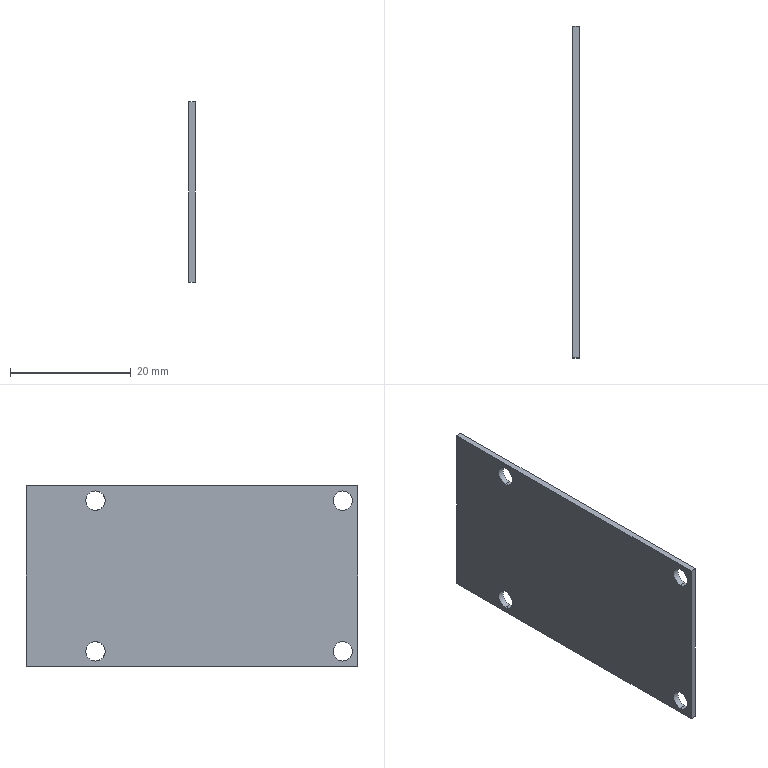Part | STEP file | RJ-GRBT-V1_1-221125 | 1 solid | 14 faces | box 1 x 55 x 30 mm | volume 1618 mm3 | cylinder 8 | plane 6 | commonest cylinder face diameters 3.2 x8
STEP:
#1=CARTESIAN_POINT('',(0.,0.,0.));
#2=DIRECTION('',(0.,0.,1.));
#3=DIRECTION('',(1.,0.,0.));
#4=AXIS2_PLACEMENT_3D('',#1,#2,#3);
#5=CARTESIAN_POINT('',(658.041,4225.2,279.644));
#6=VERTEX_POINT('',#5);
#7=CARTESIAN_POINT('',(658.041,4225.2,309.644));
#8=VERTEX_POINT('',#7);
#9=CARTESIAN_POINT('',(658.041,4225.2,279.644));
#10=DIRECTION('',(0.,0.,1.));
#11=VECTOR('',#10,1.);
#12=LINE('',#9,#11);
#13=CARTESIAN_POINT('',(659.041,4225.2,309.644));
#14=DIRECTION('',(0.,1.,0.));
#15=DIRECTION('',(0.,0.,1.));
#16=AXIS2_PLACEMENT_3D('',#13,#14,#15);
#17=PLANE('',#16);
#18=CARTESIAN_POINT('',(-30.,-1.));
#19=DIRECTION('',(1.,0.));
#20=VECTOR('',#19,1.);
#21=LINE('',#18,#20);
#22=(GEOMETRIC_REPRESENTATION_CONTEXT(2)PARAMETRIC_REPRESENTATION_CONTEXT()REPRESENTATION_CONTEXT('',''));
#23=DEFINITIONAL_REPRESENTATION('',(#21),#22);
#24=PCURVE('',#17,#23);
#25=CARTESIAN_POINT('',(658.041,4227.7,282.144));
#26=DIRECTION('',(1.,0.,0.));
#27=DIRECTION('',(0.,0.,-1.));
#28=AXIS2_PLACEMENT_3D('',#25,#26,#27);
#29=PLANE('',#28);
#30=CARTESIAN_POINT('',(2.5,-2.5));
#31=DIRECTION('',(-1.,0.));
#32=VECTOR('',#31,1.);
#33=LINE('',#30,#32);
#34=(GEOMETRIC_REPRESENTATION_CONTEXT(2)PARAMETRIC_REPRESENTATION_CONTEXT()REPRESENTATION_CONTEXT('',''));
#35=DEFINITIONAL_REPRESENTATION('',(#33),#34);
#36=PCURVE('',#29,#35);
#37=SURFACE_CURVE('',#12,(#24,#36),.PCURVE_S1.);
#38=EDGE_CURVE('',#6,#8,#37,.T.);
#39=ORIENTED_EDGE('',*,*,#38,.T.);
#40=CARTESIAN_POINT('',(659.041,4225.2,309.644));
#41=VERTEX_POINT('',#40);
#42=CARTESIAN_POINT('',(658.041,4225.2,309.644));
#43=DIRECTION('',(1.,0.,0.));
#44=VECTOR('',#43,1.);
#45=LINE('',#42,#44);
#46=CARTESIAN_POINT('',(0.,-1.));
#47=DIRECTION('',(0.,1.));
#48=VECTOR('',#47,1.);
#49=LINE('',#46,#48);
#50=(GEOMETRIC_REPRESENTATION_CONTEXT(2)PARAMETRIC_REPRESENTATION_CONTEXT()REPRESENTATION_CONTEXT('',''));
#51=DEFINITIONAL_REPRESENTATION('',(#49),#50);
#52=PCURVE('',#17,#51);
#53=CARTESIAN_POINT('',(659.041,4280.2,309.644));
#54=DIRECTION('',(0.,0.,-1.));
#55=DIRECTION('',(-1.,0.,0.));
#56=AXIS2_PLACEMENT_3D('',#53,#54,#55);
#57=PLANE('',#56);
#58=CARTESIAN_POINT('',(1.,-55.));
#59=DIRECTION('',(-1.,0.));
#60=VECTOR('',#59,1.);
#61=LINE('',#58,#60);
#62=(GEOMETRIC_REPRESENTATION_CONTEXT(2)PARAMETRIC_REPRESENTATION_CONTEXT()REPRESENTATION_CONTEXT('',''));
#63=DEFINITIONAL_REPRESENTATION('',(#61),#62);
#64=PCURVE('',#57,#63);
#65=SURFACE_CURVE('',#45,(#52,#64),.PCURVE_S1.);
#66=EDGE_CURVE('',#8,#41,#65,.T.);
#67=ORIENTED_EDGE('',*,*,#66,.T.);
#68=CARTESIAN_POINT('',(659.041,4225.2,279.644));
#69=VERTEX_POINT('',#68);
#70=CARTESIAN_POINT('',(659.041,4225.2,279.644));
#71=DIRECTION('',(0.,0.,1.));
#72=VECTOR('',#71,1.);
#73=LINE('',#70,#72);
#74=CARTESIAN_POINT('',(-30.,0.));
#75=DIRECTION('',(1.,0.));
#76=VECTOR('',#75,1.);
#77=LINE('',#74,#76);
#78=(GEOMETRIC_REPRESENTATION_CONTEXT(2)PARAMETRIC_REPRESENTATION_CONTEXT()REPRESENTATION_CONTEXT('',''));
#79=DEFINITIONAL_REPRESENTATION('',(#77),#78);
#80=PCURVE('',#17,#79);
#81=CARTESIAN_POINT('',(659.041,4227.7,282.144));
#82=DIRECTION('',(1.,0.,0.));
#83=DIRECTION('',(0.,0.,-1.));
#84=AXIS2_PLACEMENT_3D('',#81,#82,#83);
#85=PLANE('',#84);
#86=CARTESIAN_POINT('',(2.5,-2.5));
#87=DIRECTION('',(-1.,0.));
#88=VECTOR('',#87,1.);
#89=LINE('',#86,#88);
#90=(GEOMETRIC_REPRESENTATION_CONTEXT(2)PARAMETRIC_REPRESENTATION_CONTEXT()REPRESENTATION_CONTEXT('',''));
#91=DEFINITIONAL_REPRESENTATION('',(#89),#90);
#92=PCURVE('',#85,#91);
#93=SURFACE_CURVE('',#73,(#80,#92),.PCURVE_S1.);
#94=EDGE_CURVE('',#69,#41,#93,.T.);
#95=ORIENTED_EDGE('',*,*,#94,.F.);
#96=CARTESIAN_POINT('',(658.041,4225.2,279.644));
#97=DIRECTION('',(1.,0.,0.));
#98=VECTOR('',#97,1.);
#99=LINE('',#96,#98);
#100=CARTESIAN_POINT('',(-30.,-1.));
#101=DIRECTION('',(0.,1.));
#102=VECTOR('',#101,1.);
#103=LINE('',#100,#102);
#104=(GEOMETRIC_REPRESENTATION_CONTEXT(2)PARAMETRIC_REPRESENTATION_CONTEXT()REPRESENTATION_CONTEXT('',''));
#105=DEFINITIONAL_REPRESENTATION('',(#103),#104);
#106=PCURVE('',#17,#105);
#107=CARTESIAN_POINT('',(659.041,4225.2,279.644));
#108=DIRECTION('',(0.,0.,1.));
#109=DIRECTION('',(1.,0.,0.));
#110=AXIS2_PLACEMENT_3D('',#107,#108,#109);
#111=PLANE('',#110);
#112=CARTESIAN_POINT('',(-1.,0.));
#113=DIRECTION('',(1.,0.));
#114=VECTOR('',#113,1.);
#115=LINE('',#112,#114);
#116=(GEOMETRIC_REPRESENTATION_CONTEXT(2)PARAMETRIC_REPRESENTATION_CONTEXT()REPRESENTATION_CONTEXT('',''));
#117=DEFINITIONAL_REPRESENTATION('',(#115),#116);
#118=PCURVE('',#111,#117);
#119=SURFACE_CURVE('',#99,(#106,#118),.PCURVE_S1.);
#120=EDGE_CURVE('',#6,#69,#119,.T.);
#121=ORIENTED_EDGE('',*,*,#120,.F.);
#122=EDGE_LOOP('',(#39,#67,#95,#121));
#123=FACE_BOUND('',#122,.F.);
#124=ADVANCED_FACE('',(#123),#17,.F.);
#125=ORIENTED_EDGE('',*,*,#38,.F.);
#126=CARTESIAN_POINT('',(658.041,4280.2,279.644));
#127=VERTEX_POINT('',#126);
#128=CARTESIAN_POINT('',(658.041,4280.2,279.644));
#129=DIRECTION('',(0.,-1.,0.));
#130=VECTOR('',#129,1.);
#131=LINE('',#128,#130);
#132=CARTESIAN_POINT('',(2.5,52.5));
#133=DIRECTION('',(0.,-1.));
#134=VECTOR('',#133,1.);
#135=LINE('',#132,#134);
#136=(GEOMETRIC_REPRESENTATION_CONTEXT(2)PARAMETRIC_REPRESENTATION_CONTEXT()REPRESENTATION_CONTEXT('',''));
#137=DEFINITIONAL_REPRESENTATION('',(#135),#136);
#138=PCURVE('',#29,#137);
#139=CARTESIAN_POINT('',(-1.,55.));
#140=DIRECTION('',(0.,-1.));
#141=VECTOR('',#140,1.);
#142=LINE('',#139,#141);
#143=(GEOMETRIC_REPRESENTATION_CONTEXT(2)PARAMETRIC_REPRESENTATION_CONTEXT()REPRESENTATION_CONTEXT('',''));
#144=DEFINITIONAL_REPRESENTATION('',(#142),#143);
#145=PCURVE('',#111,#144);
#146=SURFACE_CURVE('',#131,(#138,#145),.PCURVE_S1.);
#147=EDGE_CURVE('',#127,#6,#146,.T.);
#148=ORIENTED_EDGE('',*,*,#147,.F.);
#149=CARTESIAN_POINT('',(658.041,4280.2,309.644));
#150=VERTEX_POINT('',#149);
#151=CARTESIAN_POINT('',(658.041,4280.2,309.644));
#152=DIRECTION('',(0.,0.,-1.));
#153=VECTOR('',#152,1.);
#154=LINE('',#151,#153);
#155=CARTESIAN_POINT('',(-27.5,52.5));
#156=DIRECTION('',(1.,0.));
#157=VECTOR('',#156,1.);
#158=LINE('',#155,#157);
#159=(GEOMETRIC_REPRESENTATION_CONTEXT(2)PARAMETRIC_REPRESENTATION_CONTEXT()REPRESENTATION_CONTEXT('',''));
#160=DEFINITIONAL_REPRESENTATION('',(#158),#159);
#161=PCURVE('',#29,#160);
#162=CARTESIAN_POINT('',(659.041,4280.2,279.644));
#163=DIRECTION('',(0.,-1.,0.));
#164=DIRECTION('',(0.,0.,-1.));
#165=AXIS2_PLACEMENT_3D('',#162,#163,#164);
#166=PLANE('',#165);
#167=CARTESIAN_POINT('',(-30.,-1.));
#168=DIRECTION('',(1.,0.));
#169=VECTOR('',#168,1.);
#170=LINE('',#167,#169);
#171=(GEOMETRIC_REPRESENTATION_CONTEXT(2)PARAMETRIC_REPRESENTATION_CONTEXT()REPRESENTATION_CONTEXT('',''));
#172=DEFINITIONAL_REPRESENTATION('',(#170),#171);
#173=PCURVE('',#166,#172);
#174=SURFACE_CURVE('',#154,(#161,#173),.PCURVE_S1.);
#175=EDGE_CURVE('',#150,#127,#174,.T.);
#176=ORIENTED_EDGE('',*,*,#175,.F.);
#177=CARTESIAN_POINT('',(658.041,4225.2,309.644));
#178=DIRECTION('',(0.,1.,0.));
#179=VECTOR('',#178,1.);
#180=LINE('',#177,#179);
#181=CARTESIAN_POINT('',(-27.5,-2.5));
#182=DIRECTION('',(0.,1.));
#183=VECTOR('',#182,1.);
#184=LINE('',#181,#183);
#185=(GEOMETRIC_REPRESENTATION_CONTEXT(2)PARAMETRIC_REPRESENTATION_CONTEXT()REPRESENTATION_CONTEXT('',''));
#186=DEFINITIONAL_REPRESENTATION('',(#184),#185);
#187=PCURVE('',#29,#186);
#188=CARTESIAN_POINT('',(1.,-55.));
#189=DIRECTION('',(0.,1.));
#190=VECTOR('',#189,1.);
#191=LINE('',#188,#190);
#192=(GEOMETRIC_REPRESENTATION_CONTEXT(2)PARAMETRIC_REPRESENTATION_CONTEXT()REPRESENTATION_CONTEXT('',''));
#193=DEFINITIONAL_REPRESENTATION('',(#191),#192);
#194=PCURVE('',#57,#193);
#195=SURFACE_CURVE('',#180,(#187,#194),.PCURVE_S1.);
#196=EDGE_CURVE('',#8,#150,#195,.T.);
#197=ORIENTED_EDGE('',*,*,#196,.F.);
#198=EDGE_LOOP('',(#125,#148,#176,#197));
#199=FACE_BOUND('',#198,.F.);
#200=CARTESIAN_POINT('',(658.041,4229.3,282.144));
#201=VERTEX_POINT('',#200);
#202=CARTESIAN_POINT('',(658.041,4227.7,283.744));
#203=VERTEX_POINT('',#202);
#204=CARTESIAN_POINT('',(658.041,4227.7,282.144));
#205=DIRECTION('',(1.,0.,0.));
#206=DIRECTION('',(0.,1.,0.));
#207=AXIS2_PLACEMENT_3D('',#204,#205,#206);
#208=CIRCLE('',#207,1.6);
#209=CARTESIAN_POINT('',(0.,0.));
#210=DIRECTION('',(0.,1.));
#211=AXIS2_PLACEMENT_2D('',#209,#210);
#212=CIRCLE('',#211,1.6);
#213=(GEOMETRIC_REPRESENTATION_CONTEXT(2)PARAMETRIC_REPRESENTATION_CONTEXT()REPRESENTATION_CONTEXT('',''));
#214=DEFINITIONAL_REPRESENTATION('',(#212),#213);
#215=PCURVE('',#29,#214);
#216=CARTESIAN_POINT('',(659.041,4227.7,282.144));
#217=DIRECTION('',(-1.,0.,0.));
#218=DIRECTION('',(0.,0.,1.));
#219=AXIS2_PLACEMENT_3D('',#216,#217,#218);
#220=CYLINDRICAL_SURFACE('',#219,1.6);
#221=CARTESIAN_POINT('',(1.571,1.));
#222=DIRECTION('',(-1.,0.));
#223=VECTOR('',#222,1.);
#224=LINE('',#221,#223);
#225=(GEOMETRIC_REPRESENTATION_CONTEXT(2)PARAMETRIC_REPRESENTATION_CONTEXT()REPRESENTATION_CONTEXT('',''));
#226=DEFINITIONAL_REPRESENTATION('',(#224),#225);
#227=PCURVE('',#220,#226);
#228=SURFACE_CURVE('',#208,(#215,#227),.PCURVE_S1.);
#229=EDGE_CURVE('',#201,#203,#228,.T.);
#230=ORIENTED_EDGE('',*,*,#229,.F.);
#231=CARTESIAN_POINT('',(658.041,4227.7,280.544));
#232=VERTEX_POINT('',#231);
#233=CARTESIAN_POINT('',(658.041,4227.7,282.144));
#234=DIRECTION('',(1.,0.,0.));
#235=DIRECTION('',(0.,0.,-1.));
#236=AXIS2_PLACEMENT_3D('',#233,#234,#235);
#237=CIRCLE('',#236,1.6);
#238=CARTESIAN_POINT('',(0.,0.));
#239=DIRECTION('',(1.,0.));
#240=AXIS2_PLACEMENT_2D('',#238,#239);
#241=CIRCLE('',#240,1.6);
#242=(GEOMETRIC_REPRESENTATION_CONTEXT(2)PARAMETRIC_REPRESENTATION_CONTEXT()REPRESENTATION_CONTEXT('',''));
#243=DEFINITIONAL_REPRESENTATION('',(#241),#242);
#244=PCURVE('',#29,#243);
#245=CARTESIAN_POINT('',(3.142,1.));
#246=DIRECTION('',(-1.,0.));
#247=VECTOR('',#246,1.);
#248=LINE('',#245,#247);
#249=(GEOMETRIC_REPRESENTATION_CONTEXT(2)PARAMETRIC_REPRESENTATION_CONTEXT()REPRESENTATION_CONTEXT('',''));
#250=DEFINITIONAL_REPRESENTATION('',(#248),#249);
#251=PCURVE('',#220,#250);
#252=SURFACE_CURVE('',#237,(#244,#251),.PCURVE_S1.);
#253=EDGE_CURVE('',#232,#201,#252,.T.);
#254=ORIENTED_EDGE('',*,*,#253,.F.);
#255=CARTESIAN_POINT('',(658.041,4226.1,282.144));
#256=VERTEX_POINT('',#255);
#257=CARTESIAN_POINT('',(658.041,4227.7,282.144));
#258=DIRECTION('',(1.,0.,0.));
#259=DIRECTION('',(0.,-1.,0.));
#260=AXIS2_PLACEMENT_3D('',#257,#258,#259);
#261=CIRCLE('',#260,1.6);
#262=CARTESIAN_POINT('',(0.,0.));
#263=DIRECTION('',(0.,-1.));
#264=AXIS2_PLACEMENT_2D('',#262,#263);
#265=CIRCLE('',#264,1.6);
#266=(GEOMETRIC_REPRESENTATION_CONTEXT(2)PARAMETRIC_REPRESENTATION_CONTEXT()REPRESENTATION_CONTEXT('',''));
#267=DEFINITIONAL_REPRESENTATION('',(#265),#266);
#268=PCURVE('',#29,#267);
#269=CARTESIAN_POINT('',(659.041,4227.7,282.144));
#270=DIRECTION('',(-1.,0.,0.));
#271=DIRECTION('',(0.,0.,1.));
#272=AXIS2_PLACEMENT_3D('',#269,#270,#271);
#273=CYLINDRICAL_SURFACE('',#272,1.6);
#274=CARTESIAN_POINT('',(4.712,1.));
#275=DIRECTION('',(-1.,0.));
#276=VECTOR('',#275,1.);
#277=LINE('',#274,#276);
#278=(GEOMETRIC_REPRESENTATION_CONTEXT(2)PARAMETRIC_REPRESENTATION_CONTEXT()REPRESENTATION_CONTEXT('',''));
#279=DEFINITIONAL_REPRESENTATION('',(#277),#278);
#280=PCURVE('',#273,#279);
#281=SURFACE_CURVE('',#261,(#268,#280),.PCURVE_S1.);
#282=EDGE_CURVE('',#256,#232,#281,.T.);
#283=ORIENTED_EDGE('',*,*,#282,.F.);
#284=CARTESIAN_POINT('',(658.041,4227.7,282.144));
#285=DIRECTION('',(1.,0.,0.));
#286=DIRECTION('',(0.,0.,1.));
#287=AXIS2_PLACEMENT_3D('',#284,#285,#286);
#288=CIRCLE('',#287,1.6);
#289=CARTESIAN_POINT('',(0.,0.));
#290=DIRECTION('',(-1.,0.));
#291=AXIS2_PLACEMENT_2D('',#289,#290);
#292=CIRCLE('',#291,1.6);
#293=(GEOMETRIC_REPRESENTATION_CONTEXT(2)PARAMETRIC_REPRESENTATION_CONTEXT()REPRESENTATION_CONTEXT('',''));
#294=DEFINITIONAL_REPRESENTATION('',(#292),#293);
#295=PCURVE('',#29,#294);
#296=CARTESIAN_POINT('',(6.283,1.));
#297=DIRECTION('',(-1.,0.));
#298=VECTOR('',#297,1.);
#299=LINE('',#296,#298);
#300=(GEOMETRIC_REPRESENTATION_CONTEXT(2)PARAMETRIC_REPRESENTATION_CONTEXT()REPRESENTATION_CONTEXT('',''));
#301=DEFINITIONAL_REPRESENTATION('',(#299),#300);
#302=PCURVE('',#273,#301);
#303=SURFACE_CURVE('',#288,(#295,#302),.PCURVE_S1.);
#304=EDGE_CURVE('',#203,#256,#303,.T.);
#305=ORIENTED_EDGE('',*,*,#304,.F.);
#306=EDGE_LOOP('',(#230,#254,#283,#305));
#307=FACE_BOUND('',#306,.F.);
#308=CARTESIAN_POINT('',(658.041,4229.3,307.144));
#309=VERTEX_POINT('',#308);
#310=CARTESIAN_POINT('',(658.041,4227.7,308.744));
#311=VERTEX_POINT('',#310);
#312=CARTESIAN_POINT('',(658.041,4227.7,307.144));
#313=DIRECTION('',(1.,0.,0.));
#314=DIRECTION('',(0.,1.,0.));
#315=AXIS2_PLACEMENT_3D('',#312,#313,#314);
#316=CIRCLE('',#315,1.6);
#317=CARTESIAN_POINT('',(-25.,0.));
#318=DIRECTION('',(0.,1.));
#319=AXIS2_PLACEMENT_2D('',#317,#318);
#320=CIRCLE('',#319,1.6);
#321=(GEOMETRIC_REPRESENTATION_CONTEXT(2)PARAMETRIC_REPRESENTATION_CONTEXT()REPRESENTATION_CONTEXT('',''));
#322=DEFINITIONAL_REPRESENTATION('',(#320),#321);
#323=PCURVE('',#29,#322);
#324=CARTESIAN_POINT('',(659.041,4227.7,307.144));
#325=DIRECTION('',(-1.,0.,0.));
#326=DIRECTION('',(0.,0.,1.));
#327=AXIS2_PLACEMENT_3D('',#324,#325,#326);
#328=CYLINDRICAL_SURFACE('',#327,1.6);
#329=CARTESIAN_POINT('',(1.571,1.));
#330=DIRECTION('',(-1.,0.));
#331=VECTOR('',#330,1.);
#332=LINE('',#329,#331);
#333=(GEOMETRIC_REPRESENTATION_CONTEXT(2)PARAMETRIC_REPRESENTATION_CONTEXT()REPRESENTATION_CONTEXT('',''));
#334=DEFINITIONAL_REPRESENTATION('',(#332),#333);
#335=PCURVE('',#328,#334);
#336=SURFACE_CURVE('',#316,(#323,#335),.PCURVE_S1.);
#337=EDGE_CURVE('',#309,#311,#336,.T.);
#338=ORIENTED_EDGE('',*,*,#337,.F.);
#339=CARTESIAN_POINT('',(658.041,4227.7,305.544));
#340=VERTEX_POINT('',#339);
#341=CARTESIAN_POINT('',(658.041,4227.7,307.144));
#342=DIRECTION('',(1.,0.,0.));
#343=DIRECTION('',(0.,0.,-1.));
#344=AXIS2_PLACEMENT_3D('',#341,#342,#343);
#345=CIRCLE('',#344,1.6);
#346=CARTESIAN_POINT('',(-25.,0.));
#347=DIRECTION('',(1.,0.));
#348=AXIS2_PLACEMENT_2D('',#346,#347);
#349=CIRCLE('',#348,1.6);
#350=(GEOMETRIC_REPRESENTATION_CONTEXT(2)PARAMETRIC_REPRESENTATION_CONTEXT()REPRESENTATION_CONTEXT('',''));
#351=DEFINITIONAL_REPRESENTATION('',(#349),#350);
#352=PCURVE('',#29,#351);
#353=CARTESIAN_POINT('',(3.142,1.));
#354=DIRECTION('',(-1.,0.));
#355=VECTOR('',#354,1.);
#356=LINE('',#353,#355);
#357=(GEOMETRIC_REPRESENTATION_CONTEXT(2)PARAMETRIC_REPRESENTATION_CONTEXT()REPRESENTATION_CONTEXT('',''));
#358=DEFINITIONAL_REPRESENTATION('',(#356),#357);
#359=PCURVE('',#328,#358);
#360=SURFACE_CURVE('',#345,(#352,#359),.PCURVE_S1.);
#361=EDGE_CURVE('',#340,#309,#360,.T.);
#362=ORIENTED_EDGE('',*,*,#361,.F.);
#363=CARTESIAN_POINT('',(658.041,4226.1,307.144));
#364=VERTEX_POINT('',#363);
#365=CARTESIAN_POINT('',(658.041,4227.7,307.144));
#366=DIRECTION('',(1.,0.,0.));
#367=DIRECTION('',(0.,-1.,0.));
#368=AXIS2_PLACEMENT_3D('',#365,#366,#367);
#369=CIRCLE('',#368,1.6);
#370=CARTESIAN_POINT('',(-25.,0.));
#371=DIRECTION('',(0.,-1.));
#372=AXIS2_PLACEMENT_2D('',#370,#371);
#373=CIRCLE('',#372,1.6);
#374=(GEOMETRIC_REPRESENTATION_CONTEXT(2)PARAMETRIC_REPRESENTATION_CONTEXT()REPRESENTATION_CONTEXT('',''));
#375=DEFINITIONAL_REPRESENTATION('',(#373),#374);
#376=PCURVE('',#29,#375);
#377=CARTESIAN_POINT('',(659.041,4227.7,307.144));
#378=DIRECTION('',(-1.,0.,0.));
#379=DIRECTION('',(0.,0.,1.));
#380=AXIS2_PLACEMENT_3D('',#377,#378,#379);
#381=CYLINDRICAL_SURFACE('',#380,1.6);
#382=CARTESIAN_POINT('',(4.712,1.));
#383=DIRECTION('',(-1.,0.));
#384=VECTOR('',#383,1.);
#385=LINE('',#382,#384);
#386=(GEOMETRIC_REPRESENTATION_CONTEXT(2)PARAMETRIC_REPRESENTATION_CONTEXT()REPRESENTATION_CONTEXT('',''));
#387=DEFINITIONAL_REPRESENTATION('',(#385),#386);
#388=PCURVE('',#381,#387);
#389=SURFACE_CURVE('',#369,(#376,#388),.PCURVE_S1.);
#390=EDGE_CURVE('',#364,#340,#389,.T.);
#391=ORIENTED_EDGE('',*,*,#390,.F.);
#392=CARTESIAN_POINT('',(658.041,4227.7,307.144));
#393=DIRECTION('',(1.,0.,0.));
#394=DIRECTION('',(0.,0.,1.));
#395=AXIS2_PLACEMENT_3D('',#392,#393,#394);
#396=CIRCLE('',#395,1.6);
#397=CARTESIAN_POINT('',(-25.,0.));
#398=DIRECTION('',(-1.,0.));
#399=AXIS2_PLACEMENT_2D('',#397,#398);
#400=CIRCLE('',#399,1.6);
#401=(GEOMETRIC_REPRESENTATION_CONTEXT(2)PARAMETRIC_REPRESENTATION_CONTEXT()REPRESENTATION_CONTEXT('',''));
#402=DEFINITIONAL_REPRESENTATION('',(#400),#401);
#403=PCURVE('',#29,#402);
#404=CARTESIAN_POINT('',(6.283,1.));
#405=DIRECTION('',(-1.,0.));
#406=VECTOR('',#405,1.);
#407=LINE('',#404,#406);
#408=(GEOMETRIC_REPRESENTATION_CONTEXT(2)PARAMETRIC_REPRESENTATION_CONTEXT()REPRESENTATION_CONTEXT('',''));
#409=DEFINITIONAL_REPRESENTATION('',(#407),#408);
#410=PCURVE('',#381,#409);
#411=SURFACE_CURVE('',#396,(#403,#410),.PCURVE_S1.);
#412=EDGE_CURVE('',#311,#364,#411,.T.);
#413=ORIENTED_EDGE('',*,*,#412,.F.);
#414=EDGE_LOOP('',(#338,#362,#391,#413));
#415=FACE_BOUND('',#414,.F.);
#416=CARTESIAN_POINT('',(658.041,4270.3,282.144));
#417=VERTEX_POINT('',#416);
#418=CARTESIAN_POINT('',(658.041,4268.7,283.744));
#419=VERTEX_POINT('',#418);
#420=CARTESIAN_POINT('',(658.041,4268.7,282.144));
#421=DIRECTION('',(1.,0.,0.));
#422=DIRECTION('',(0.,1.,0.));
#423=AXIS2_PLACEMENT_3D('',#420,#421,#422);
#424=CIRCLE('',#423,1.6);
#425=CARTESIAN_POINT('',(0.,41.));
#426=DIRECTION('',(0.,1.));
#427=AXIS2_PLACEMENT_2D('',#425,#426);
#428=CIRCLE('',#427,1.6);
#429=(GEOMETRIC_REPRESENTATION_CONTEXT(2)PARAMETRIC_REPRESENTATION_CONTEXT()REPRESENTATION_CONTEXT('',''));
#430=DEFINITIONAL_REPRESENTATION('',(#428),#429);
#431=PCURVE('',#29,#430);
#432=CARTESIAN_POINT('',(659.041,4268.7,282.144));
#433=DIRECTION('',(-1.,0.,0.));
#434=DIRECTION('',(0.,0.,1.));
#435=AXIS2_PLACEMENT_3D('',#432,#433,#434);
#436=CYLINDRICAL_SURFACE('',#435,1.6);
#437=CARTESIAN_POINT('',(1.571,1.));
#438=DIRECTION('',(-1.,0.));
#439=VECTOR('',#438,1.);
#440=LINE('',#437,#439);
#441=(GEOMETRIC_REPRESENTATION_CONTEXT(2)PARAMETRIC_REPRESENTATION_CONTEXT()REPRESENTATION_CONTEXT('',''));
#442=DEFINITIONAL_REPRESENTATION('',(#440),#441);
#443=PCURVE('',#436,#442);
#444=SURFACE_CURVE('',#424,(#431,#443),.PCURVE_S1.);
#445=EDGE_CURVE('',#417,#419,#444,.T.);
#446=ORIENTED_EDGE('',*,*,#445,.F.);
#447=CARTESIAN_POINT('',(658.041,4268.7,280.544));
#448=VERTEX_POINT('',#447);
#449=CARTESIAN_POINT('',(658.041,4268.7,282.144));
#450=DIRECTION('',(1.,0.,0.));
#451=DIRECTION('',(0.,0.,-1.));
#452=AXIS2_PLACEMENT_3D('',#449,#450,#451);
#453=CIRCLE('',#452,1.6);
#454=CARTESIAN_POINT('',(0.,41.));
#455=DIRECTION('',(1.,0.));
#456=AXIS2_PLACEMENT_2D('',#454,#455);
#457=CIRCLE('',#456,1.6);
#458=(GEOMETRIC_REPRESENTATION_CONTEXT(2)PARAMETRIC_REPRESENTATION_CONTEXT()REPRESENTATION_CONTEXT('',''));
#459=DEFINITIONAL_REPRESENTATION('',(#457),#458);
#460=PCURVE('',#29,#459);
#461=CARTESIAN_POINT('',(3.142,1.));
#462=DIRECTION('',(-1.,0.));
#463=VECTOR('',#462,1.);
#464=LINE('',#461,#463);
#465=(GEOMETRIC_REPRESENTATION_CONTEXT(2)PARAMETRIC_REPRESENTATION_CONTEXT()REPRESENTATION_CONTEXT('',''));
#466=DEFINITIONAL_REPRESENTATION('',(#464),#465);
#467=PCURVE('',#436,#466);
#468=SURFACE_CURVE('',#453,(#460,#467),.PCURVE_S1.);
#469=EDGE_CURVE('',#448,#417,#468,.T.);
#470=ORIENTED_EDGE('',*,*,#469,.F.);
#471=CARTESIAN_POINT('',(658.041,4267.1,282.144));
#472=VERTEX_POINT('',#471);
#473=CARTESIAN_POINT('',(658.041,4268.7,282.144));
#474=DIRECTION('',(1.,0.,0.));
#475=DIRECTION('',(0.,-1.,0.));
#476=AXIS2_PLACEMENT_3D('',#473,#474,#475);
#477=CIRCLE('',#476,1.6);
#478=CARTESIAN_POINT('',(0.,41.));
#479=DIRECTION('',(0.,-1.));
#480=AXIS2_PLACEMENT_2D('',#478,#479);
#481=CIRCLE('',#480,1.6);
#482=(GEOMETRIC_REPRESENTATION_CONTEXT(2)PARAMETRIC_REPRESENTATION_CONTEXT()REPRESENTATION_CONTEXT('',''));
#483=DEFINITIONAL_REPRESENTATION('',(#481),#482);
#484=PCURVE('',#29,#483);
#485=CARTESIAN_POINT('',(659.041,4268.7,282.144));
#486=DIRECTION('',(-1.,0.,0.));
#487=DIRECTION('',(0.,0.,1.));
#488=AXIS2_PLACEMENT_3D('',#485,#486,#487);
#489=CYLINDRICAL_SURFACE('',#488,1.6);
#490=CARTESIAN_POINT('',(4.712,1.));
#491=DIRECTION('',(-1.,0.));
#492=VECTOR('',#491,1.);
#493=LINE('',#490,#492);
#494=(GEOMETRIC_REPRESENTATION_CONTEXT(2)PARAMETRIC_REPRESENTATION_CONTEXT()REPRESENTATION_CONTEXT('',''));
#495=DEFINITIONAL_REPRESENTATION('',(#493),#494);
#496=PCURVE('',#489,#495);
#497=SURFACE_CURVE('',#477,(#484,#496),.PCURVE_S1.);
#498=EDGE_CURVE('',#472,#448,#497,.T.);
#499=ORIENTED_EDGE('',*,*,#498,.F.);
#500=CARTESIAN_POINT('',(658.041,4268.7,282.144));
#501=DIRECTION('',(1.,0.,0.));
#502=DIRECTION('',(0.,0.,1.));
#503=AXIS2_PLACEMENT_3D('',#500,#501,#502);
#504=CIRCLE('',#503,1.6);
#505=CARTESIAN_POINT('',(0.,41.));
#506=DIRECTION('',(-1.,0.));
#507=AXIS2_PLACEMENT_2D('',#505,#506);
#508=CIRCLE('',#507,1.6);
#509=(GEOMETRIC_REPRESENTATION_CONTEXT(2)PARAMETRIC_REPRESENTATION_CONTEXT()REPRESENTATION_CONTEXT('',''));
#510=DEFINITIONAL_REPRESENTATION('',(#508),#509);
#511=PCURVE('',#29,#510);
#512=CARTESIAN_POINT('',(6.283,1.));
#513=DIRECTION('',(-1.,0.));
#514=VECTOR('',#513,1.);
#515=LINE('',#512,#514);
#516=(GEOMETRIC_REPRESENTATION_CONTEXT(2)PARAMETRIC_REPRESENTATION_CONTEXT()REPRESENTATION_CONTEXT('',''));
#517=DEFINITIONAL_REPRESENTATION('',(#515),#516);
#518=PCURVE('',#489,#517);
#519=SURFACE_CURVE('',#504,(#511,#518),.PCURVE_S1.);
#520=EDGE_CURVE('',#419,#472,#519,.T.);
#521=ORIENTED_EDGE('',*,*,#520,.F.);
#522=EDGE_LOOP('',(#446,#470,#499,#521));
#523=FACE_BOUND('',#522,.F.);
#524=CARTESIAN_POINT('',(658.041,4270.3,307.144));
#525=VERTEX_POINT('',#524);
#526=CARTESIAN_POINT('',(658.041,4268.7,308.744));
#527=VERTEX_POINT('',#526);
#528=CARTESIAN_POINT('',(658.041,4268.7,307.144));
#529=DIRECTION('',(1.,0.,0.));
#530=DIRECTION('',(0.,1.,0.));
#531=AXIS2_PLACEMENT_3D('',#528,#529,#530);
#532=CIRCLE('',#531,1.6);
#533=CARTESIAN_POINT('',(-25.,41.));
#534=DIRECTION('',(0.,1.));
#535=AXIS2_PLACEMENT_2D('',#533,#534);
#536=CIRCLE('',#535,1.6);
#537=(GEOMETRIC_REPRESENTATION_CONTEXT(2)PARAMETRIC_REPRESENTATION_CONTEXT()REPRESENTATION_CONTEXT('',''));
#538=DEFINITIONAL_REPRESENTATION('',(#536),#537);
#539=PCURVE('',#29,#538);
#540=CARTESIAN_POINT('',(659.041,4268.7,307.144));
#541=DIRECTION('',(-1.,0.,0.));
#542=DIRECTION('',(0.,0.,1.));
#543=AXIS2_PLACEMENT_3D('',#540,#541,#542);
#544=CYLINDRICAL_SURFACE('',#543,1.6);
#545=CARTESIAN_POINT('',(1.571,1.));
#546=DIRECTION('',(-1.,0.));
#547=VECTOR('',#546,1.);
#548=LINE('',#545,#547);
#549=(GEOMETRIC_REPRESENTATION_CONTEXT(2)PARAMETRIC_REPRESENTATION_CONTEXT()REPRESENTATION_CONTEXT('',''));
#550=DEFINITIONAL_REPRESENTATION('',(#548),#549);
#551=PCURVE('',#544,#550);
#552=SURFACE_CURVE('',#532,(#539,#551),.PCURVE_S1.);
#553=EDGE_CURVE('',#525,#527,#552,.T.);
#554=ORIENTED_EDGE('',*,*,#553,.F.);
#555=CARTESIAN_POINT('',(658.041,4268.7,305.544));
#556=VERTEX_POINT('',#555);
#557=CARTESIAN_POINT('',(658.041,4268.7,307.144));
#558=DIRECTION('',(1.,0.,0.));
#559=DIRECTION('',(0.,0.,-1.));
#560=AXIS2_PLACEMENT_3D('',#557,#558,#559);
#561=CIRCLE('',#560,1.6);
#562=CARTESIAN_POINT('',(-25.,41.));
#563=DIRECTION('',(1.,0.));
#564=AXIS2_PLACEMENT_2D('',#562,#563);
#565=CIRCLE('',#564,1.6);
#566=(GEOMETRIC_REPRESENTATION_CONTEXT(2)PARAMETRIC_REPRESENTATION_CONTEXT()REPRESENTATION_CONTEXT('',''));
#567=DEFINITIONAL_REPRESENTATION('',(#565),#566);
#568=PCURVE('',#29,#567);
#569=CARTESIAN_POINT('',(3.142,1.));
#570=DIRECTION('',(-1.,0.));
#571=VECTOR('',#570,1.);
#572=LINE('',#569,#571);
#573=(GEOMETRIC_REPRESENTATION_CONTEXT(2)PARAMETRIC_REPRESENTATION_CONTEXT()REPRESENTATION_CONTEXT('',''));
#574=DEFINITIONAL_REPRESENTATION('',(#572),#573);
#575=PCURVE('',#544,#574);
#576=SURFACE_CURVE('',#561,(#568,#575),.PCURVE_S1.);
#577=EDGE_CURVE('',#556,#525,#576,.T.);
#578=ORIENTED_EDGE('',*,*,#577,.F.);
#579=CARTESIAN_POINT('',(658.041,4267.1,307.144));
#580=VERTEX_POINT('',#579);
#581=CARTESIAN_POINT('',(658.041,4268.7,307.144));
#582=DIRECTION('',(1.,0.,0.));
#583=DIRECTION('',(0.,-1.,0.));
#584=AXIS2_PLACEMENT_3D('',#581,#582,#583);
#585=CIRCLE('',#584,1.6);
#586=CARTESIAN_POINT('',(-25.,41.));
#587=DIRECTION('',(0.,-1.));
#588=AXIS2_PLACEMENT_2D('',#586,#587);
#589=CIRCLE('',#588,1.6);
#590=(GEOMETRIC_REPRESENTATION_CONTEXT(2)PARAMETRIC_REPRESENTATION_CONTEXT()REPRESENTATION_CONTEXT('',''));
#591=DEFINITIONAL_REPRESENTATION('',(#589),#590);
#592=PCURVE('',#29,#591);
#593=CARTESIAN_POINT('',(659.041,4268.7,307.144));
#594=DIRECTION('',(-1.,0.,0.));
#595=DIRECTION('',(0.,0.,1.));
#596=AXIS2_PLACEMENT_3D('',#593,#594,#595);
#597=CYLINDRICAL_SURFACE('',#596,1.6);
#598=CARTESIAN_POINT('',(4.712,1.));
#599=DIRECTION('',(-1.,0.));
#600=VECTOR('',#599,1.);
#601=LINE('',#598,#600);
#602=(GEOMETRIC_REPRESENTATION_CONTEXT(2)PARAMETRIC_REPRESENTATION_CONTEXT()REPRESENTATION_CONTEXT('',''));
#603=DEFINITIONAL_REPRESENTATION('',(#601),#602);
#604=PCURVE('',#597,#603);
#605=SURFACE_CURVE('',#585,(#592,#604),.PCURVE_S1.);
#606=EDGE_CURVE('',#580,#556,#605,.T.);
#607=ORIENTED_EDGE('',*,*,#606,.F.);
#608=CARTESIAN_POINT('',(658.041,4268.7,307.144));
#609=DIRECTION('',(1.,0.,0.));
#610=DIRECTION('',(0.,0.,1.));
#611=AXIS2_PLACEMENT_3D('',#608,#609,#610);
#612=CIRCLE('',#611,1.6);
#613=CARTESIAN_POINT('',(-25.,41.));
#614=DIRECTION('',(-1.,0.));
#615=AXIS2_PLACEMENT_2D('',#613,#614);
#616=CIRCLE('',#615,1.6);
#617=(GEOMETRIC_REPRESENTATION_CONTEXT(2)PARAMETRIC_REPRESENTATION_CONTEXT()REPRESENTATION_CONTEXT('',''));
#618=DEFINITIONAL_REPRESENTATION('',(#616),#617);
#619=PCURVE('',#29,#618);
#620=CARTESIAN_POINT('',(6.283,1.));
#621=DIRECTION('',(-1.,0.));
#622=VECTOR('',#621,1.);
#623=LINE('',#620,#622);
#624=(GEOMETRIC_REPRESENTATION_CONTEXT(2)PARAMETRIC_REPRESENTATION_CONTEXT()REPRESENTATION_CONTEXT('',''));
#625=DEFINITIONAL_REPRESENTATION('',(#623),#624);
#626=PCURVE('',#597,#625);
#627=SURFACE_CURVE('',#612,(#619,#626),.PCURVE_S1.);
#628=EDGE_CURVE('',#527,#580,#627,.T.);
#629=ORIENTED_EDGE('',*,*,#628,.F.);
#630=EDGE_LOOP('',(#554,#578,#607,#629));
#631=FACE_BOUND('',#630,.F.);
#632=ADVANCED_FACE('',(#199,#307,#415,#523,#631),#29,.F.);
#633=ORIENTED_EDGE('',*,*,#147,.T.);
#634=ORIENTED_EDGE('',*,*,#120,.T.);
#635=CARTESIAN_POINT('',(659.041,4280.2,279.644));
#636=VERTEX_POINT('',#635);
#637=CARTESIAN_POINT('',(659.041,4280.2,279.644));
#638=DIRECTION('',(0.,-1.,0.));
#639=VECTOR('',#638,1.);
#640=LINE('',#637,#639);
#641=CARTESIAN_POINT('',(0.,55.));
#642=DIRECTION('',(0.,-1.));
#643=VECTOR('',#642,1.);
#644=LINE('',#641,#643);
#645=(GEOMETRIC_REPRESENTATION_CONTEXT(2)PARAMETRIC_REPRESENTATION_CONTEXT()REPRESENTATION_CONTEXT('',''));
#646=DEFINITIONAL_REPRESENTATION('',(#644),#645);
#647=PCURVE('',#111,#646);
#648=CARTESIAN_POINT('',(2.5,52.5));
#649=DIRECTION('',(0.,-1.));
#650=VECTOR('',#649,1.);
#651=LINE('',#648,#650);
#652=(GEOMETRIC_REPRESENTATION_CONTEXT(2)PARAMETRIC_REPRESENTATION_CONTEXT()REPRESENTATION_CONTEXT('',''));
#653=DEFINITIONAL_REPRESENTATION('',(#651),#652);
#654=PCURVE('',#85,#653);
#655=SURFACE_CURVE('',#640,(#647,#654),.PCURVE_S1.);
#656=EDGE_CURVE('',#636,#69,#655,.T.);
#657=ORIENTED_EDGE('',*,*,#656,.F.);
#658=CARTESIAN_POINT('',(658.041,4280.2,279.644));
#659=DIRECTION('',(1.,0.,0.));
#660=VECTOR('',#659,1.);
#661=LINE('',#658,#660);
#662=CARTESIAN_POINT('',(-1.,55.));
#663=DIRECTION('',(1.,0.));
#664=VECTOR('',#663,1.);
#665=LINE('',#662,#664);
#666=(GEOMETRIC_REPRESENTATION_CONTEXT(2)PARAMETRIC_REPRESENTATION_CONTEXT()REPRESENTATION_CONTEXT('',''));
#667=DEFINITIONAL_REPRESENTATION('',(#665),#666);
#668=PCURVE('',#111,#667);
#669=CARTESIAN_POINT('',(0.,-1.));
#670=DIRECTION('',(0.,1.));
#671=VECTOR('',#670,1.);
#672=LINE('',#669,#671);
#673=(GEOMETRIC_REPRESENTATION_CONTEXT(2)PARAMETRIC_REPRESENTATION_CONTEXT()REPRESENTATION_CONTEXT('',''));
#674=DEFINITIONAL_REPRESENTATION('',(#672),#673);
#675=PCURVE('',#166,#674);
#676=SURFACE_CURVE('',#661,(#668,#675),.PCURVE_S1.);
#677=EDGE_CURVE('',#127,#636,#676,.T.);
#678=ORIENTED_EDGE('',*,*,#677,.F.);
#679=EDGE_LOOP('',(#633,#634,#657,#678));
#680=FACE_BOUND('',#679,.F.);
#681=ADVANCED_FACE('',(#680),#111,.F.);
#682=ORIENTED_EDGE('',*,*,#94,.T.);
#683=CARTESIAN_POINT('',(659.041,4280.2,309.644));
#684=VERTEX_POINT('',#683);
#685=CARTESIAN_POINT('',(659.041,4225.2,309.644));
#686=DIRECTION('',(0.,1.,0.));
#687=VECTOR('',#686,1.);
#688=LINE('',#685,#687);
#689=CARTESIAN_POINT('',(-27.5,-2.5));
#690=DIRECTION('',(0.,1.));
#691=VECTOR('',#690,1.);
#692=LINE('',#689,#691);
#693=(GEOMETRIC_REPRESENTATION_CONTEXT(2)PARAMETRIC_REPRESENTATION_CONTEXT()REPRESENTATION_CONTEXT('',''));
#694=DEFINITIONAL_REPRESENTATION('',(#692),#693);
#695=PCURVE('',#85,#694);
#696=CARTESIAN_POINT('',(0.,-55.));
#697=DIRECTION('',(0.,1.));
#698=VECTOR('',#697,1.);
#699=LINE('',#696,#698);
#700=(GEOMETRIC_REPRESENTATION_CONTEXT(2)PARAMETRIC_REPRESENTATION_CONTEXT()REPRESENTATION_CONTEXT('',''));
#701=DEFINITIONAL_REPRESENTATION('',(#699),#700);
#702=PCURVE('',#57,#701);
#703=SURFACE_CURVE('',#688,(#695,#702),.PCURVE_S1.);
#704=EDGE_CURVE('',#41,#684,#703,.T.);
#705=ORIENTED_EDGE('',*,*,#704,.T.);
#706=CARTESIAN_POINT('',(659.041,4280.2,309.644));
#707=DIRECTION('',(0.,0.,-1.));
#708=VECTOR('',#707,1.);
#709=LINE('',#706,#708);
#710=CARTESIAN_POINT('',(-27.5,52.5));
#711=DIRECTION('',(1.,0.));
#712=VECTOR('',#711,1.);
#713=LINE('',#710,#712);
#714=(GEOMETRIC_REPRESENTATION_CONTEXT(2)PARAMETRIC_REPRESENTATION_CONTEXT()REPRESENTATION_CONTEXT('',''));
#715=DEFINITIONAL_REPRESENTATION('',(#713),#714);
#716=PCURVE('',#85,#715);
#717=CARTESIAN_POINT('',(-30.,0.));
#718=DIRECTION('',(1.,0.));
#719=VECTOR('',#718,1.);
#720=LINE('',#717,#719);
#721=(GEOMETRIC_REPRESENTATION_CONTEXT(2)PARAMETRIC_REPRESENTATION_CONTEXT()REPRESENTATION_CONTEXT('',''));
#722=DEFINITIONAL_REPRESENTATION('',(#720),#721);
#723=PCURVE('',#166,#722);
#724=SURFACE_CURVE('',#709,(#716,#723),.PCURVE_S1.);
#725=EDGE_CURVE('',#684,#636,#724,.T.);
#726=ORIENTED_EDGE('',*,*,#725,.T.);
#727=ORIENTED_EDGE('',*,*,#656,.T.);
#728=EDGE_LOOP('',(#682,#705,#726,#727));
#729=FACE_BOUND('',#728,.F.);
#730=CARTESIAN_POINT('',(659.041,4229.3,282.144));
#731=VERTEX_POINT('',#730);
#732=CARTESIAN_POINT('',(659.041,4227.7,280.544));
#733=VERTEX_POINT('',#732);
#734=CARTESIAN_POINT('',(659.041,4227.7,282.144));
#735=DIRECTION('',(-1.,0.,0.));
#736=DIRECTION('',(0.,1.,0.));
#737=AXIS2_PLACEMENT_3D('',#734,#735,#736);
#738=CIRCLE('',#737,1.6);
#739=CARTESIAN_POINT('',(0.,1.6));
#740=CARTESIAN_POINT('',(2.771,1.6));
#741=CARTESIAN_POINT('',(1.386,-0.8));
#742=CARTESIAN_POINT('',(0.,-3.2));
#743=CARTESIAN_POINT('',(-1.386,-0.8));
#744=CARTESIAN_POINT('',(-2.771,1.6));
#745=CARTESIAN_POINT('',(0.,1.6));
#746=(BOUNDED_CURVE()B_SPLINE_CURVE(2,(#739,#740,#741,#742,#743,#744,#745),.UNSPECIFIED.,.T.,.F.)B_SPLINE_CURVE_WITH_KNOTS((1,2,2,2,2,1),(-2.094,0.,2.094,4.189,6.283,8.378),.UNSPECIFIED.)CURVE()GEOMETRIC_REPRESENTATION_ITEM()RATIONAL_B_SPLINE_CURVE((1.,0.5,1.,0.5,1.,0.5,1.))REPRESENTATION_ITEM(''));
#747=(GEOMETRIC_REPRESENTATION_CONTEXT(2)PARAMETRIC_REPRESENTATION_CONTEXT()REPRESENTATION_CONTEXT('',''));
#748=DEFINITIONAL_REPRESENTATION('',(#746),#747);
#749=PCURVE('',#85,#748);
#750=CARTESIAN_POINT('',(1.571,0.));
#751=DIRECTION('',(1.,0.));
#752=VECTOR('',#751,1.);
#753=LINE('',#750,#752);
#754=(GEOMETRIC_REPRESENTATION_CONTEXT(2)PARAMETRIC_REPRESENTATION_CONTEXT()REPRESENTATION_CONTEXT('',''));
#755=DEFINITIONAL_REPRESENTATION('',(#753),#754);
#756=PCURVE('',#220,#755);
#757=SURFACE_CURVE('',#738,(#749,#756),.PCURVE_S1.);
#758=EDGE_CURVE('',#731,#733,#757,.T.);
#759=ORIENTED_EDGE('',*,*,#758,.F.);
#760=CARTESIAN_POINT('',(659.041,4227.7,283.744));
#761=VERTEX_POINT('',#760);
#762=CARTESIAN_POINT('',(659.041,4227.7,282.144));
#763=DIRECTION('',(-1.,0.,0.));
#764=DIRECTION('',(0.,0.,1.));
#765=AXIS2_PLACEMENT_3D('',#762,#763,#764);
#766=CIRCLE('',#765,1.6);
#767=CARTESIAN_POINT('',(-1.6,0.));
#768=CARTESIAN_POINT('',(-1.6,2.771));
#769=CARTESIAN_POINT('',(0.8,1.386));
#770=CARTESIAN_POINT('',(3.2,0.));
#771=CARTESIAN_POINT('',(0.8,-1.386));
#772=CARTESIAN_POINT('',(-1.6,-2.771));
#773=CARTESIAN_POINT('',(-1.6,0.));
#774=(BOUNDED_CURVE()B_SPLINE_CURVE(2,(#767,#768,#769,#770,#771,#772,#773),.UNSPECIFIED.,.T.,.F.)B_SPLINE_CURVE_WITH_KNOTS((1,2,2,2,2,1),(-2.094,0.,2.094,4.189,6.283,8.378),.UNSPECIFIED.)CURVE()GEOMETRIC_REPRESENTATION_ITEM()RATIONAL_B_SPLINE_CURVE((1.,0.5,1.,0.5,1.,0.5,1.))REPRESENTATION_ITEM(''));
#775=(GEOMETRIC_REPRESENTATION_CONTEXT(2)PARAMETRIC_REPRESENTATION_CONTEXT()REPRESENTATION_CONTEXT('',''));
#776=DEFINITIONAL_REPRESENTATION('',(#774),#775);
#777=PCURVE('',#85,#776);
#778=CARTESIAN_POINT('',(0.,0.));
#779=DIRECTION('',(1.,0.));
#780=VECTOR('',#779,1.);
#781=LINE('',#778,#780);
#782=(GEOMETRIC_REPRESENTATION_CONTEXT(2)PARAMETRIC_REPRESENTATION_CONTEXT()REPRESENTATION_CONTEXT('',''));
#783=DEFINITIONAL_REPRESENTATION('',(#781),#782);
#784=PCURVE('',#220,#783);
#785=SURFACE_CURVE('',#766,(#777,#784),.PCURVE_S1.);
#786=EDGE_CURVE('',#761,#731,#785,.T.);
#787=ORIENTED_EDGE('',*,*,#786,.F.);
#788=CARTESIAN_POINT('',(659.041,4227.7,282.144));
#789=DIRECTION('',(-1.,0.,0.));
#790=DIRECTION('',(0.,0.,-1.));
#791=AXIS2_PLACEMENT_3D('',#788,#789,#790);
#792=CIRCLE('',#791,1.6);
#793=CARTESIAN_POINT('',(1.6,0.));
#794=CARTESIAN_POINT('',(1.6,-2.771));
#795=CARTESIAN_POINT('',(-0.8,-1.386));
#796=CARTESIAN_POINT('',(-3.2,0.));
#797=CARTESIAN_POINT('',(-0.8,1.386));
#798=CARTESIAN_POINT('',(1.6,2.771));
#799=CARTESIAN_POINT('',(1.6,0.));
#800=(BOUNDED_CURVE()B_SPLINE_CURVE(2,(#793,#794,#795,#796,#797,#798,#799),.UNSPECIFIED.,.T.,.F.)B_SPLINE_CURVE_WITH_KNOTS((1,2,2,2,2,1),(-2.094,0.,2.094,4.189,6.283,8.378),.UNSPECIFIED.)CURVE()GEOMETRIC_REPRESENTATION_ITEM()RATIONAL_B_SPLINE_CURVE((1.,0.5,1.,0.5,1.,0.5,1.))REPRESENTATION_ITEM(''));
#801=(GEOMETRIC_REPRESENTATION_CONTEXT(2)PARAMETRIC_REPRESENTATION_CONTEXT()REPRESENTATION_CONTEXT('',''));
#802=DEFINITIONAL_REPRESENTATION('',(#800),#801);
#803=PCURVE('',#85,#802);
#804=CARTESIAN_POINT('',(3.142,0.));
#805=DIRECTION('',(1.,0.));
#806=VECTOR('',#805,1.);
#807=LINE('',#804,#806);
#808=(GEOMETRIC_REPRESENTATION_CONTEXT(2)PARAMETRIC_REPRESENTATION_CONTEXT()REPRESENTATION_CONTEXT('',''));
#809=DEFINITIONAL_REPRESENTATION('',(#807),#808);
#810=PCURVE('',#273,#809);
#811=SURFACE_CURVE('',#792,(#803,#810),.PCURVE_S1.);
#812=EDGE_CURVE('',#733,#761,#811,.T.);
#813=ORIENTED_EDGE('',*,*,#812,.F.);
#814=EDGE_LOOP('',(#759,#787,#813));
#815=FACE_BOUND('',#814,.F.);
#816=CARTESIAN_POINT('',(659.041,4229.3,307.144));
#817=VERTEX_POINT('',#816);
#818=CARTESIAN_POINT('',(659.041,4227.7,305.544));
#819=VERTEX_POINT('',#818);
#820=CARTESIAN_POINT('',(659.041,4227.7,307.144));
#821=DIRECTION('',(-1.,0.,0.));
#822=DIRECTION('',(0.,1.,0.));
#823=AXIS2_PLACEMENT_3D('',#820,#821,#822);
#824=CIRCLE('',#823,1.6);
#825=CARTESIAN_POINT('',(-25.,1.6));
#826=CARTESIAN_POINT('',(-22.229,1.6));
#827=CARTESIAN_POINT('',(-23.614,-0.8));
#828=CARTESIAN_POINT('',(-25.,-3.2));
#829=CARTESIAN_POINT('',(-26.386,-0.8));
#830=CARTESIAN_POINT('',(-27.771,1.6));
#831=CARTESIAN_POINT('',(-25.,1.6));
#832=(BOUNDED_CURVE()B_SPLINE_CURVE(2,(#825,#826,#827,#828,#829,#830,#831),.UNSPECIFIED.,.T.,.F.)B_SPLINE_CURVE_WITH_KNOTS((1,2,2,2,2,1),(-2.094,0.,2.094,4.189,6.283,8.378),.UNSPECIFIED.)CURVE()GEOMETRIC_REPRESENTATION_ITEM()RATIONAL_B_SPLINE_CURVE((1.,0.5,1.,0.5,1.,0.5,1.))REPRESENTATION_ITEM(''));
#833=(GEOMETRIC_REPRESENTATION_CONTEXT(2)PARAMETRIC_REPRESENTATION_CONTEXT()REPRESENTATION_CONTEXT('',''));
#834=DEFINITIONAL_REPRESENTATION('',(#832),#833);
#835=PCURVE('',#85,#834);
#836=CARTESIAN_POINT('',(1.571,0.));
#837=DIRECTION('',(1.,0.));
#838=VECTOR('',#837,1.);
#839=LINE('',#836,#838);
#840=(GEOMETRIC_REPRESENTATION_CONTEXT(2)PARAMETRIC_REPRESENTATION_CONTEXT()REPRESENTATION_CONTEXT('',''));
#841=DEFINITIONAL_REPRESENTATION('',(#839),#840);
#842=PCURVE('',#328,#841);
#843=SURFACE_CURVE('',#824,(#835,#842),.PCURVE_S1.);
#844=EDGE_CURVE('',#817,#819,#843,.T.);
#845=ORIENTED_EDGE('',*,*,#844,.F.);
#846=CARTESIAN_POINT('',(659.041,4227.7,308.744));
#847=VERTEX_POINT('',#846);
#848=CARTESIAN_POINT('',(659.041,4227.7,307.144));
#849=DIRECTION('',(-1.,0.,0.));
#850=DIRECTION('',(0.,0.,1.));
#851=AXIS2_PLACEMENT_3D('',#848,#849,#850);
#852=CIRCLE('',#851,1.6);
#853=CARTESIAN_POINT('',(-26.6,0.));
#854=CARTESIAN_POINT('',(-26.6,2.771));
#855=CARTESIAN_POINT('',(-24.2,1.386));
#856=CARTESIAN_POINT('',(-21.8,0.));
#857=CARTESIAN_POINT('',(-24.2,-1.386));
#858=CARTESIAN_POINT('',(-26.6,-2.771));
#859=CARTESIAN_POINT('',(-26.6,0.));
#860=(BOUNDED_CURVE()B_SPLINE_CURVE(2,(#853,#854,#855,#856,#857,#858,#859),.UNSPECIFIED.,.T.,.F.)B_SPLINE_CURVE_WITH_KNOTS((1,2,2,2,2,1),(-2.094,0.,2.094,4.189,6.283,8.378),.UNSPECIFIED.)CURVE()GEOMETRIC_REPRESENTATION_ITEM()RATIONAL_B_SPLINE_CURVE((1.,0.5,1.,0.5,1.,0.5,1.))REPRESENTATION_ITEM(''));
#861=(GEOMETRIC_REPRESENTATION_CONTEXT(2)PARAMETRIC_REPRESENTATION_CONTEXT()REPRESENTATION_CONTEXT('',''));
#862=DEFINITIONAL_REPRESENTATION('',(#860),#861);
#863=PCURVE('',#85,#862);
#864=CARTESIAN_POINT('',(0.,0.));
#865=DIRECTION('',(1.,0.));
#866=VECTOR('',#865,1.);
#867=LINE('',#864,#866);
#868=(GEOMETRIC_REPRESENTATION_CONTEXT(2)PARAMETRIC_REPRESENTATION_CONTEXT()REPRESENTATION_CONTEXT('',''));
#869=DEFINITIONAL_REPRESENTATION('',(#867),#868);
#870=PCURVE('',#328,#869);
#871=SURFACE_CURVE('',#852,(#863,#870),.PCURVE_S1.);
#872=EDGE_CURVE('',#847,#817,#871,.T.);
#873=ORIENTED_EDGE('',*,*,#872,.F.);
#874=CARTESIAN_POINT('',(659.041,4227.7,307.144));
#875=DIRECTION('',(-1.,0.,0.));
#876=DIRECTION('',(0.,0.,-1.));
#877=AXIS2_PLACEMENT_3D('',#874,#875,#876);
#878=CIRCLE('',#877,1.6);
#879=CARTESIAN_POINT('',(-23.4,0.));
#880=CARTESIAN_POINT('',(-23.4,-2.771));
#881=CARTESIAN_POINT('',(-25.8,-1.386));
#882=CARTESIAN_POINT('',(-28.2,0.));
#883=CARTESIAN_POINT('',(-25.8,1.386));
#884=CARTESIAN_POINT('',(-23.4,2.771));
#885=CARTESIAN_POINT('',(-23.4,0.));
#886=(BOUNDED_CURVE()B_SPLINE_CURVE(2,(#879,#880,#881,#882,#883,#884,#885),.UNSPECIFIED.,.T.,.F.)B_SPLINE_CURVE_WITH_KNOTS((1,2,2,2,2,1),(-2.094,0.,2.094,4.189,6.283,8.378),.UNSPECIFIED.)CURVE()GEOMETRIC_REPRESENTATION_ITEM()RATIONAL_B_SPLINE_CURVE((1.,0.5,1.,0.5,1.,0.5,1.))REPRESENTATION_ITEM(''));
#887=(GEOMETRIC_REPRESENTATION_CONTEXT(2)PARAMETRIC_REPRESENTATION_CONTEXT()REPRESENTATION_CONTEXT('',''));
#888=DEFINITIONAL_REPRESENTATION('',(#886),#887);
#889=PCURVE('',#85,#888);
#890=CARTESIAN_POINT('',(3.142,0.));
#891=DIRECTION('',(1.,0.));
#892=VECTOR('',#891,1.);
#893=LINE('',#890,#892);
#894=(GEOMETRIC_REPRESENTATION_CONTEXT(2)PARAMETRIC_REPRESENTATION_CONTEXT()REPRESENTATION_CONTEXT('',''));
#895=DEFINITIONAL_REPRESENTATION('',(#893),#894);
#896=PCURVE('',#381,#895);
#897=SURFACE_CURVE('',#878,(#889,#896),.PCURVE_S1.);
#898=EDGE_CURVE('',#819,#847,#897,.T.);
#899=ORIENTED_EDGE('',*,*,#898,.F.);
#900=EDGE_LOOP('',(#845,#873,#899));
#901=FACE_BOUND('',#900,.F.);
#902=CARTESIAN_POINT('',(659.041,4270.3,282.144));
#903=VERTEX_POINT('',#902);
#904=CARTESIAN_POINT('',(659.041,4268.7,280.544));
#905=VERTEX_POINT('',#904);
#906=CARTESIAN_POINT('',(659.041,4268.7,282.144));
#907=DIRECTION('',(-1.,0.,0.));
#908=DIRECTION('',(0.,1.,0.));
#909=AXIS2_PLACEMENT_3D('',#906,#907,#908);
#910=CIRCLE('',#909,1.6);
#911=CARTESIAN_POINT('',(0.,42.6));
#912=CARTESIAN_POINT('',(2.771,42.6));
#913=CARTESIAN_POINT('',(1.386,40.2));
#914=CARTESIAN_POINT('',(0.,37.8));
#915=CARTESIAN_POINT('',(-1.386,40.2));
#916=CARTESIAN_POINT('',(-2.771,42.6));
#917=CARTESIAN_POINT('',(0.,42.6));
#918=(BOUNDED_CURVE()B_SPLINE_CURVE(2,(#911,#912,#913,#914,#915,#916,#917),.UNSPECIFIED.,.T.,.F.)B_SPLINE_CURVE_WITH_KNOTS((1,2,2,2,2,1),(-2.094,0.,2.094,4.189,6.283,8.378),.UNSPECIFIED.)CURVE()GEOMETRIC_REPRESENTATION_ITEM()RATIONAL_B_SPLINE_CURVE((1.,0.5,1.,0.5,1.,0.5,1.))REPRESENTATION_ITEM(''));
#919=(GEOMETRIC_REPRESENTATION_CONTEXT(2)PARAMETRIC_REPRESENTATION_CONTEXT()REPRESENTATION_CONTEXT('',''));
#920=DEFINITIONAL_REPRESENTATION('',(#918),#919);
#921=PCURVE('',#85,#920);
#922=CARTESIAN_POINT('',(1.571,0.));
#923=DIRECTION('',(1.,0.));
#924=VECTOR('',#923,1.);
#925=LINE('',#922,#924);
#926=(GEOMETRIC_REPRESENTATION_CONTEXT(2)PARAMETRIC_REPRESENTATION_CONTEXT()REPRESENTATION_CONTEXT('',''));
#927=DEFINITIONAL_REPRESENTATION('',(#925),#926);
#928=PCURVE('',#436,#927);
#929=SURFACE_CURVE('',#910,(#921,#928),.PCURVE_S1.);
#930=EDGE_CURVE('',#903,#905,#929,.T.);
#931=ORIENTED_EDGE('',*,*,#930,.F.);
#932=CARTESIAN_POINT('',(659.041,4268.7,283.744));
#933=VERTEX_POINT('',#932);
#934=CARTESIAN_POINT('',(659.041,4268.7,282.144));
#935=DIRECTION('',(-1.,0.,0.));
#936=DIRECTION('',(0.,0.,1.));
#937=AXIS2_PLACEMENT_3D('',#934,#935,#936);
#938=CIRCLE('',#937,1.6);
#939=CARTESIAN_POINT('',(-1.6,41.));
#940=CARTESIAN_POINT('',(-1.6,43.771));
#941=CARTESIAN_POINT('',(0.8,42.386));
#942=CARTESIAN_POINT('',(3.2,41.));
#943=CARTESIAN_POINT('',(0.8,39.614));
#944=CARTESIAN_POINT('',(-1.6,38.229));
#945=CARTESIAN_POINT('',(-1.6,41.));
#946=(BOUNDED_CURVE()B_SPLINE_CURVE(2,(#939,#940,#941,#942,#943,#944,#945),.UNSPECIFIED.,.T.,.F.)B_SPLINE_CURVE_WITH_KNOTS((1,2,2,2,2,1),(-2.094,0.,2.094,4.189,6.283,8.378),.UNSPECIFIED.)CURVE()GEOMETRIC_REPRESENTATION_ITEM()RATIONAL_B_SPLINE_CURVE((1.,0.5,1.,0.5,1.,0.5,1.))REPRESENTATION_ITEM(''));
#947=(GEOMETRIC_REPRESENTATION_CONTEXT(2)PARAMETRIC_REPRESENTATION_CONTEXT()REPRESENTATION_CONTEXT('',''));
#948=DEFINITIONAL_REPRESENTATION('',(#946),#947);
#949=PCURVE('',#85,#948);
#950=CARTESIAN_POINT('',(0.,0.));
#951=DIRECTION('',(1.,0.));
#952=VECTOR('',#951,1.);
#953=LINE('',#950,#952);
#954=(GEOMETRIC_REPRESENTATION_CONTEXT(2)PARAMETRIC_REPRESENTATION_CONTEXT()REPRESENTATION_CONTEXT('',''));
#955=DEFINITIONAL_REPRESENTATION('',(#953),#954);
#956=PCURVE('',#436,#955);
#957=SURFACE_CURVE('',#938,(#949,#956),.PCURVE_S1.);
#958=EDGE_CURVE('',#933,#903,#957,.T.);
#959=ORIENTED_EDGE('',*,*,#958,.F.);
#960=CARTESIAN_POINT('',(659.041,4268.7,282.144));
#961=DIRECTION('',(-1.,0.,0.));
#962=DIRECTION('',(0.,0.,-1.));
#963=AXIS2_PLACEMENT_3D('',#960,#961,#962);
#964=CIRCLE('',#963,1.6);
#965=CARTESIAN_POINT('',(1.6,41.));
#966=CARTESIAN_POINT('',(1.6,38.229));
#967=CARTESIAN_POINT('',(-0.8,39.614));
#968=CARTESIAN_POINT('',(-3.2,41.));
#969=CARTESIAN_POINT('',(-0.8,42.386));
#970=CARTESIAN_POINT('',(1.6,43.771));
#971=CARTESIAN_POINT('',(1.6,41.));
#972=(BOUNDED_CURVE()B_SPLINE_CURVE(2,(#965,#966,#967,#968,#969,#970,#971),.UNSPECIFIED.,.T.,.F.)B_SPLINE_CURVE_WITH_KNOTS((1,2,2,2,2,1),(-2.094,0.,2.094,4.189,6.283,8.378),.UNSPECIFIED.)CURVE()GEOMETRIC_REPRESENTATION_ITEM()RATIONAL_B_SPLINE_CURVE((1.,0.5,1.,0.5,1.,0.5,1.))REPRESENTATION_ITEM(''));
#973=(GEOMETRIC_REPRESENTATION_CONTEXT(2)PARAMETRIC_REPRESENTATION_CONTEXT()REPRESENTATION_CONTEXT('',''));
#974=DEFINITIONAL_REPRESENTATION('',(#972),#973);
#975=PCURVE('',#85,#974);
#976=CARTESIAN_POINT('',(3.142,0.));
#977=DIRECTION('',(1.,0.));
#978=VECTOR('',#977,1.);
#979=LINE('',#976,#978);
#980=(GEOMETRIC_REPRESENTATION_CONTEXT(2)PARAMETRIC_REPRESENTATION_CONTEXT()REPRESENTATION_CONTEXT('',''));
#981=DEFINITIONAL_REPRESENTATION('',(#979),#980);
#982=PCURVE('',#489,#981);
#983=SURFACE_CURVE('',#964,(#975,#982),.PCURVE_S1.);
#984=EDGE_CURVE('',#905,#933,#983,.T.);
#985=ORIENTED_EDGE('',*,*,#984,.F.);
#986=EDGE_LOOP('',(#931,#959,#985));
#987=FACE_BOUND('',#986,.F.);
#988=CARTESIAN_POINT('',(659.041,4270.3,307.144));
#989=VERTEX_POINT('',#988);
#990=CARTESIAN_POINT('',(659.041,4268.7,305.544));
#991=VERTEX_POINT('',#990);
#992=CARTESIAN_POINT('',(659.041,4268.7,307.144));
#993=DIRECTION('',(-1.,0.,0.));
#994=DIRECTION('',(0.,1.,0.));
#995=AXIS2_PLACEMENT_3D('',#992,#993,#994);
#996=CIRCLE('',#995,1.6);
#997=CARTESIAN_POINT('',(-25.,42.6));
#998=CARTESIAN_POINT('',(-22.229,42.6));
#999=CARTESIAN_POINT('',(-23.614,40.2));
#1000=CARTESIAN_POINT('',(-25.,37.8));
#1001=CARTESIAN_POINT('',(-26.386,40.2));
#1002=CARTESIAN_POINT('',(-27.771,42.6));
#1003=CARTESIAN_POINT('',(-25.,42.6));
#1004=(BOUNDED_CURVE()B_SPLINE_CURVE(2,(#997,#998,#999,#1000,#1001,#1002,#1003),.UNSPECIFIED.,.T.,.F.)B_SPLINE_CURVE_WITH_KNOTS((1,2,2,2,2,1),(-2.094,0.,2.094,4.189,6.283,8.378),.UNSPECIFIED.)CURVE()GEOMETRIC_REPRESENTATION_ITEM()RATIONAL_B_SPLINE_CURVE((1.,0.5,1.,0.5,1.,0.5,1.))REPRESENTATION_ITEM(''));
#1005=(GEOMETRIC_REPRESENTATION_CONTEXT(2)PARAMETRIC_REPRESENTATION_CONTEXT()REPRESENTATION_CONTEXT('',''));
#1006=DEFINITIONAL_REPRESENTATION('',(#1004),#1005);
#1007=PCURVE('',#85,#1006);
#1008=CARTESIAN_POINT('',(1.571,0.));
#1009=DIRECTION('',(1.,0.));
#1010=VECTOR('',#1009,1.);
#1011=LINE('',#1008,#1010);
#1012=(GEOMETRIC_REPRESENTATION_CONTEXT(2)PARAMETRIC_REPRESENTATION_CONTEXT()REPRESENTATION_CONTEXT('',''));
#1013=DEFINITIONAL_REPRESENTATION('',(#1011),#1012);
#1014=PCURVE('',#544,#1013);
#1015=SURFACE_CURVE('',#996,(#1007,#1014),.PCURVE_S1.);
#1016=EDGE_CURVE('',#989,#991,#1015,.T.);
#1017=ORIENTED_EDGE('',*,*,#1016,.F.);
#1018=CARTESIAN_POINT('',(659.041,4268.7,308.744));
#1019=VERTEX_POINT('',#1018);
#1020=CARTESIAN_POINT('',(659.041,4268.7,307.144));
#1021=DIRECTION('',(-1.,0.,0.));
#1022=DIRECTION('',(0.,0.,1.));
#1023=AXIS2_PLACEMENT_3D('',#1020,#1021,#1022);
#1024=CIRCLE('',#1023,1.6);
#1025=CARTESIAN_POINT('',(-26.6,41.));
#1026=CARTESIAN_POINT('',(-26.6,43.771));
#1027=CARTESIAN_POINT('',(-24.2,42.386));
#1028=CARTESIAN_POINT('',(-21.8,41.));
#1029=CARTESIAN_POINT('',(-24.2,39.614));
#1030=CARTESIAN_POINT('',(-26.6,38.229));
#1031=CARTESIAN_POINT('',(-26.6,41.));
#1032=(BOUNDED_CURVE()B_SPLINE_CURVE(2,(#1025,#1026,#1027,#1028,#1029,#1030,#1031),.UNSPECIFIED.,.T.,.F.)B_SPLINE_CURVE_WITH_KNOTS((1,2,2,2,2,1),(-2.094,0.,2.094,4.189,6.283,8.378),.UNSPECIFIED.)CURVE()GEOMETRIC_REPRESENTATION_ITEM()RATIONAL_B_SPLINE_CURVE((1.,0.5,1.,0.5,1.,0.5,1.))REPRESENTATION_ITEM(''));
#1033=(GEOMETRIC_REPRESENTATION_CONTEXT(2)PARAMETRIC_REPRESENTATION_CONTEXT()REPRESENTATION_CONTEXT('',''));
#1034=DEFINITIONAL_REPRESENTATION('',(#1032),#1033);
#1035=PCURVE('',#85,#1034);
#1036=CARTESIAN_POINT('',(0.,0.));
#1037=DIRECTION('',(1.,0.));
#1038=VECTOR('',#1037,1.);
#1039=LINE('',#1036,#1038);
#1040=(GEOMETRIC_REPRESENTATION_CONTEXT(2)PARAMETRIC_REPRESENTATION_CONTEXT()REPRESENTATION_CONTEXT('',''));
#1041=DEFINITIONAL_REPRESENTATION('',(#1039),#1040);
#1042=PCURVE('',#544,#1041);
#1043=SURFACE_CURVE('',#1024,(#1035,#1042),.PCURVE_S1.);
#1044=EDGE_CURVE('',#1019,#989,#1043,.T.);
#1045=ORIENTED_EDGE('',*,*,#1044,.F.);
#1046=CARTESIAN_POINT('',(659.041,4268.7,307.144));
#1047=DIRECTION('',(-1.,0.,0.));
#1048=DIRECTION('',(0.,0.,-1.));
#1049=AXIS2_PLACEMENT_3D('',#1046,#1047,#1048);
#1050=CIRCLE('',#1049,1.6);
#1051=CARTESIAN_POINT('',(-23.4,41.));
#1052=CARTESIAN_POINT('',(-23.4,38.229));
#1053=CARTESIAN_POINT('',(-25.8,39.614));
#1054=CARTESIAN_POINT('',(-28.2,41.));
#1055=CARTESIAN_POINT('',(-25.8,42.386));
#1056=CARTESIAN_POINT('',(-23.4,43.771));
#1057=CARTESIAN_POINT('',(-23.4,41.));
#1058=(BOUNDED_CURVE()B_SPLINE_CURVE(2,(#1051,#1052,#1053,#1054,#1055,#1056,#1057),.UNSPECIFIED.,.T.,.F.)B_SPLINE_CURVE_WITH_KNOTS((1,2,2,2,2,1),(-2.094,0.,2.094,4.189,6.283,8.378),.UNSPECIFIED.)CURVE()GEOMETRIC_REPRESENTATION_ITEM()RATIONAL_B_SPLINE_CURVE((1.,0.5,1.,0.5,1.,0.5,1.))REPRESENTATION_ITEM(''));
#1059=(GEOMETRIC_REPRESENTATION_CONTEXT(2)PARAMETRIC_REPRESENTATION_CONTEXT()REPRESENTATION_CONTEXT('',''));
#1060=DEFINITIONAL_REPRESENTATION('',(#1058),#1059);
#1061=PCURVE('',#85,#1060);
#1062=CARTESIAN_POINT('',(3.142,0.));
#1063=DIRECTION('',(1.,0.));
#1064=VECTOR('',#1063,1.);
#1065=LINE('',#1062,#1064);
#1066=(GEOMETRIC_REPRESENTATION_CONTEXT(2)PARAMETRIC_REPRESENTATION_CONTEXT()REPRESENTATION_CONTEXT('',''));
#1067=DEFINITIONAL_REPRESENTATION('',(#1065),#1066);
#1068=PCURVE('',#597,#1067);
#1069=SURFACE_CURVE('',#1050,(#1061,#1068),.PCURVE_S1.);
#1070=EDGE_CURVE('',#991,#1019,#1069,.T.);
#1071=ORIENTED_EDGE('',*,*,#1070,.F.);
#1072=EDGE_LOOP('',(#1017,#1045,#1071));
#1073=FACE_BOUND('',#1072,.F.);
#1074=ADVANCED_FACE('',(#729,#815,#901,#987,#1073),#85,.T.);
#1075=ORIENTED_EDGE('',*,*,#196,.T.);
#1076=CARTESIAN_POINT('',(658.041,4280.2,309.644));
#1077=DIRECTION('',(1.,0.,0.));
#1078=VECTOR('',#1077,1.);
#1079=LINE('',#1076,#1078);
#1080=CARTESIAN_POINT('',(1.,0.));
#1081=DIRECTION('',(-1.,0.));
#1082=VECTOR('',#1081,1.);
#1083=LINE('',#1080,#1082);
#1084=(GEOMETRIC_REPRESENTATION_CONTEXT(2)PARAMETRIC_REPRESENTATION_CONTEXT()REPRESENTATION_CONTEXT('',''));
#1085=DEFINITIONAL_REPRESENTATION('',(#1083),#1084);
#1086=PCURVE('',#57,#1085);
#1087=CARTESIAN_POINT('',(-30.,-1.));
#1088=DIRECTION('',(0.,1.));
#1089=VECTOR('',#1088,1.);
#1090=LINE('',#1087,#1089);
#1091=(GEOMETRIC_REPRESENTATION_CONTEXT(2)PARAMETRIC_REPRESENTATION_CONTEXT()REPRESENTATION_CONTEXT('',''));
#1092=DEFINITIONAL_REPRESENTATION('',(#1090),#1091);
#1093=PCURVE('',#166,#1092);
#1094=SURFACE_CURVE('',#1079,(#1086,#1093),.PCURVE_S1.);
#1095=EDGE_CURVE('',#150,#684,#1094,.T.);
#1096=ORIENTED_EDGE('',*,*,#1095,.T.);
#1097=ORIENTED_EDGE('',*,*,#704,.F.);
#1098=ORIENTED_EDGE('',*,*,#66,.F.);
#1099=EDGE_LOOP('',(#1075,#1096,#1097,#1098));
#1100=FACE_BOUND('',#1099,.F.);
#1101=ADVANCED_FACE('',(#1100),#57,.F.);
#1102=ORIENTED_EDGE('',*,*,#175,.T.);
#1103=ORIENTED_EDGE('',*,*,#677,.T.);
#1104=ORIENTED_EDGE('',*,*,#725,.F.);
#1105=ORIENTED_EDGE('',*,*,#1095,.F.);
#1106=EDGE_LOOP('',(#1102,#1103,#1104,#1105));
#1107=FACE_BOUND('',#1106,.F.);
#1108=ADVANCED_FACE('',(#1107),#166,.F.);
#1109=ORIENTED_EDGE('',*,*,#786,.T.);
#1110=ORIENTED_EDGE('',*,*,#758,.T.);
#1111=CARTESIAN_POINT('',(659.041,4227.7,280.544));
#1112=DIRECTION('',(-1.,0.,0.));
#1113=VECTOR('',#1112,1.);
#1114=LINE('',#1111,#1113);
#1115=CARTESIAN_POINT('',(3.142,0.));
#1116=DIRECTION('',(0.,1.));
#1117=VECTOR('',#1116,1.);
#1118=LINE('',#1115,#1117);
#1119=(GEOMETRIC_REPRESENTATION_CONTEXT(2)PARAMETRIC_REPRESENTATION_CONTEXT()REPRESENTATION_CONTEXT('',''));
#1120=DEFINITIONAL_REPRESENTATION('',(#1118),#1119);
#1121=PCURVE('',#220,#1120);
#1122=CARTESIAN_POINT('',(3.142,0.));
#1123=DIRECTION('',(0.,1.));
#1124=VECTOR('',#1123,1.);
#1125=LINE('',#1122,#1124);
#1126=(GEOMETRIC_REPRESENTATION_CONTEXT(2)PARAMETRIC_REPRESENTATION_CONTEXT()REPRESENTATION_CONTEXT('',''));
#1127=DEFINITIONAL_REPRESENTATION('',(#1125),#1126);
#1128=PCURVE('',#273,#1127);
#1129=SURFACE_CURVE('',#1114,(#1121,#1128),.PCURVE_S1.);
#1130=EDGE_CURVE('',#733,#232,#1129,.T.);
#1131=ORIENTED_EDGE('',*,*,#1130,.T.);
#1132=ORIENTED_EDGE('',*,*,#253,.T.);
#1133=ORIENTED_EDGE('',*,*,#229,.T.);
#1134=CARTESIAN_POINT('',(659.041,4227.7,283.744));
#1135=DIRECTION('',(-1.,0.,0.));
#1136=VECTOR('',#1135,1.);
#1137=LINE('',#1134,#1136);
#1138=CARTESIAN_POINT('',(0.,0.));
#1139=DIRECTION('',(0.,1.));
#1140=VECTOR('',#1139,1.);
#1141=LINE('',#1138,#1140);
#1142=(GEOMETRIC_REPRESENTATION_CONTEXT(2)PARAMETRIC_REPRESENTATION_CONTEXT()REPRESENTATION_CONTEXT('',''));
#1143=DEFINITIONAL_REPRESENTATION('',(#1141),#1142);
#1144=PCURVE('',#220,#1143);
#1145=CARTESIAN_POINT('',(6.283,0.));
#1146=DIRECTION('',(0.,1.));
#1147=VECTOR('',#1146,1.);
#1148=LINE('',#1145,#1147);
#1149=(GEOMETRIC_REPRESENTATION_CONTEXT(2)PARAMETRIC_REPRESENTATION_CONTEXT()REPRESENTATION_CONTEXT('',''));
#1150=DEFINITIONAL_REPRESENTATION('',(#1148),#1149);
#1151=PCURVE('',#273,#1150);
#1152=SURFACE_CURVE('',#1137,(#1144,#1151),.PCURVE_S1.);
#1153=EDGE_CURVE('',#761,#203,#1152,.T.);
#1154=ORIENTED_EDGE('',*,*,#1153,.F.);
#1155=EDGE_LOOP('',(#1109,#1110,#1131,#1132,#1133,#1154));
#1156=FACE_BOUND('',#1155,.F.);
#1157=ADVANCED_FACE('',(#1156),#220,.F.);
#1158=ORIENTED_EDGE('',*,*,#812,.T.);
#1159=ORIENTED_EDGE('',*,*,#1153,.T.);
#1160=ORIENTED_EDGE('',*,*,#304,.T.);
#1161=ORIENTED_EDGE('',*,*,#282,.T.);
#1162=ORIENTED_EDGE('',*,*,#1130,.F.);
#1163=EDGE_LOOP('',(#1158,#1159,#1160,#1161,#1162));
#1164=FACE_BOUND('',#1163,.F.);
#1165=ADVANCED_FACE('',(#1164),#273,.F.);
#1166=ORIENTED_EDGE('',*,*,#872,.T.);
#1167=ORIENTED_EDGE('',*,*,#844,.T.);
#1168=CARTESIAN_POINT('',(659.041,4227.7,305.544));
#1169=DIRECTION('',(-1.,0.,0.));
#1170=VECTOR('',#1169,1.);
#1171=LINE('',#1168,#1170);
#1172=CARTESIAN_POINT('',(3.142,0.));
#1173=DIRECTION('',(0.,1.));
#1174=VECTOR('',#1173,1.);
#1175=LINE('',#1172,#1174);
#1176=(GEOMETRIC_REPRESENTATION_CONTEXT(2)PARAMETRIC_REPRESENTATION_CONTEXT()REPRESENTATION_CONTEXT('',''));
#1177=DEFINITIONAL_REPRESENTATION('',(#1175),#1176);
#1178=PCURVE('',#328,#1177);
#1179=CARTESIAN_POINT('',(3.142,0.));
#1180=DIRECTION('',(0.,1.));
#1181=VECTOR('',#1180,1.);
#1182=LINE('',#1179,#1181);
#1183=(GEOMETRIC_REPRESENTATION_CONTEXT(2)PARAMETRIC_REPRESENTATION_CONTEXT()REPRESENTATION_CONTEXT('',''));
#1184=DEFINITIONAL_REPRESENTATION('',(#1182),#1183);
#1185=PCURVE('',#381,#1184);
#1186=SURFACE_CURVE('',#1171,(#1178,#1185),.PCURVE_S1.);
#1187=EDGE_CURVE('',#819,#340,#1186,.T.);
#1188=ORIENTED_EDGE('',*,*,#1187,.T.);
#1189=ORIENTED_EDGE('',*,*,#361,.T.);
#1190=ORIENTED_EDGE('',*,*,#337,.T.);
#1191=CARTESIAN_POINT('',(659.041,4227.7,308.744));
#1192=DIRECTION('',(-1.,0.,0.));
#1193=VECTOR('',#1192,1.);
#1194=LINE('',#1191,#1193);
#1195=CARTESIAN_POINT('',(0.,0.));
#1196=DIRECTION('',(0.,1.));
#1197=VECTOR('',#1196,1.);
#1198=LINE('',#1195,#1197);
#1199=(GEOMETRIC_REPRESENTATION_CONTEXT(2)PARAMETRIC_REPRESENTATION_CONTEXT()REPRESENTATION_CONTEXT('',''));
#1200=DEFINITIONAL_REPRESENTATION('',(#1198),#1199);
#1201=PCURVE('',#328,#1200);
#1202=CARTESIAN_POINT('',(6.283,0.));
#1203=DIRECTION('',(0.,1.));
#1204=VECTOR('',#1203,1.);
#1205=LINE('',#1202,#1204);
#1206=(GEOMETRIC_REPRESENTATION_CONTEXT(2)PARAMETRIC_REPRESENTATION_CONTEXT()REPRESENTATION_CONTEXT('',''));
#1207=DEFINITIONAL_REPRESENTATION('',(#1205),#1206);
#1208=PCURVE('',#381,#1207);
#1209=SURFACE_CURVE('',#1194,(#1201,#1208),.PCURVE_S1.);
#1210=EDGE_CURVE('',#847,#311,#1209,.T.);
#1211=ORIENTED_EDGE('',*,*,#1210,.F.);
#1212=EDGE_LOOP('',(#1166,#1167,#1188,#1189,#1190,#1211));
#1213=FACE_BOUND('',#1212,.F.);
#1214=ADVANCED_FACE('',(#1213),#328,.F.);
#1215=ORIENTED_EDGE('',*,*,#898,.T.);
#1216=ORIENTED_EDGE('',*,*,#1210,.T.);
#1217=ORIENTED_EDGE('',*,*,#412,.T.);
#1218=ORIENTED_EDGE('',*,*,#390,.T.);
#1219=ORIENTED_EDGE('',*,*,#1187,.F.);
#1220=EDGE_LOOP('',(#1215,#1216,#1217,#1218,#1219));
#1221=FACE_BOUND('',#1220,.F.);
#1222=ADVANCED_FACE('',(#1221),#381,.F.);
#1223=ORIENTED_EDGE('',*,*,#958,.T.);
#1224=ORIENTED_EDGE('',*,*,#930,.T.);
#1225=CARTESIAN_POINT('',(659.041,4268.7,280.544));
#1226=DIRECTION('',(-1.,0.,0.));
#1227=VECTOR('',#1226,1.);
#1228=LINE('',#1225,#1227);
#1229=CARTESIAN_POINT('',(3.142,0.));
#1230=DIRECTION('',(0.,1.));
#1231=VECTOR('',#1230,1.);
#1232=LINE('',#1229,#1231);
#1233=(GEOMETRIC_REPRESENTATION_CONTEXT(2)PARAMETRIC_REPRESENTATION_CONTEXT()REPRESENTATION_CONTEXT('',''));
#1234=DEFINITIONAL_REPRESENTATION('',(#1232),#1233);
#1235=PCURVE('',#436,#1234);
#1236=CARTESIAN_POINT('',(3.142,0.));
#1237=DIRECTION('',(0.,1.));
#1238=VECTOR('',#1237,1.);
#1239=LINE('',#1236,#1238);
#1240=(GEOMETRIC_REPRESENTATION_CONTEXT(2)PARAMETRIC_REPRESENTATION_CONTEXT()REPRESENTATION_CONTEXT('',''));
#1241=DEFINITIONAL_REPRESENTATION('',(#1239),#1240);
#1242=PCURVE('',#489,#1241);
#1243=SURFACE_CURVE('',#1228,(#1235,#1242),.PCURVE_S1.);
#1244=EDGE_CURVE('',#905,#448,#1243,.T.);
#1245=ORIENTED_EDGE('',*,*,#1244,.T.);
#1246=ORIENTED_EDGE('',*,*,#469,.T.);
#1247=ORIENTED_EDGE('',*,*,#445,.T.);
#1248=CARTESIAN_POINT('',(659.041,4268.7,283.744));
#1249=DIRECTION('',(-1.,0.,0.));
#1250=VECTOR('',#1249,1.);
#1251=LINE('',#1248,#1250);
#1252=CARTESIAN_POINT('',(0.,0.));
#1253=DIRECTION('',(0.,1.));
#1254=VECTOR('',#1253,1.);
#1255=LINE('',#1252,#1254);
#1256=(GEOMETRIC_REPRESENTATION_CONTEXT(2)PARAMETRIC_REPRESENTATION_CONTEXT()REPRESENTATION_CONTEXT('',''));
#1257=DEFINITIONAL_REPRESENTATION('',(#1255),#1256);
#1258=PCURVE('',#436,#1257);
#1259=CARTESIAN_POINT('',(6.283,0.));
#1260=DIRECTION('',(0.,1.));
#1261=VECTOR('',#1260,1.);
#1262=LINE('',#1259,#1261);
#1263=(GEOMETRIC_REPRESENTATION_CONTEXT(2)PARAMETRIC_REPRESENTATION_CONTEXT()REPRESENTATION_CONTEXT('',''));
#1264=DEFINITIONAL_REPRESENTATION('',(#1262),#1263);
#1265=PCURVE('',#489,#1264);
#1266=SURFACE_CURVE('',#1251,(#1258,#1265),.PCURVE_S1.);
#1267=EDGE_CURVE('',#933,#419,#1266,.T.);
#1268=ORIENTED_EDGE('',*,*,#1267,.F.);
#1269=EDGE_LOOP('',(#1223,#1224,#1245,#1246,#1247,#1268));
#1270=FACE_BOUND('',#1269,.F.);
#1271=ADVANCED_FACE('',(#1270),#436,.F.);
#1272=ORIENTED_EDGE('',*,*,#984,.T.);
#1273=ORIENTED_EDGE('',*,*,#1267,.T.);
#1274=ORIENTED_EDGE('',*,*,#520,.T.);
#1275=ORIENTED_EDGE('',*,*,#498,.T.);
#1276=ORIENTED_EDGE('',*,*,#1244,.F.);
#1277=EDGE_LOOP('',(#1272,#1273,#1274,#1275,#1276));
#1278=FACE_BOUND('',#1277,.F.);
#1279=ADVANCED_FACE('',(#1278),#489,.F.);
#1280=ORIENTED_EDGE('',*,*,#1044,.T.);
#1281=ORIENTED_EDGE('',*,*,#1016,.T.);
#1282=CARTESIAN_POINT('',(659.041,4268.7,305.544));
#1283=DIRECTION('',(-1.,0.,0.));
#1284=VECTOR('',#1283,1.);
#1285=LINE('',#1282,#1284);
#1286=CARTESIAN_POINT('',(3.142,0.));
#1287=DIRECTION('',(0.,1.));
#1288=VECTOR('',#1287,1.);
#1289=LINE('',#1286,#1288);
#1290=(GEOMETRIC_REPRESENTATION_CONTEXT(2)PARAMETRIC_REPRESENTATION_CONTEXT()REPRESENTATION_CONTEXT('',''));
#1291=DEFINITIONAL_REPRESENTATION('',(#1289),#1290);
#1292=PCURVE('',#544,#1291);
#1293=CARTESIAN_POINT('',(3.142,0.));
#1294=DIRECTION('',(0.,1.));
#1295=VECTOR('',#1294,1.);
#1296=LINE('',#1293,#1295);
#1297=(GEOMETRIC_REPRESENTATION_CONTEXT(2)PARAMETRIC_REPRESENTATION_CONTEXT()REPRESENTATION_CONTEXT('',''));
#1298=DEFINITIONAL_REPRESENTATION('',(#1296),#1297);
#1299=PCURVE('',#597,#1298);
#1300=SURFACE_CURVE('',#1285,(#1292,#1299),.PCURVE_S1.);
#1301=EDGE_CURVE('',#991,#556,#1300,.T.);
#1302=ORIENTED_EDGE('',*,*,#1301,.T.);
#1303=ORIENTED_EDGE('',*,*,#577,.T.);
#1304=ORIENTED_EDGE('',*,*,#553,.T.);
#1305=CARTESIAN_POINT('',(659.041,4268.7,308.744));
#1306=DIRECTION('',(-1.,0.,0.));
#1307=VECTOR('',#1306,1.);
#1308=LINE('',#1305,#1307);
#1309=CARTESIAN_POINT('',(0.,0.));
#1310=DIRECTION('',(0.,1.));
#1311=VECTOR('',#1310,1.);
#1312=LINE('',#1309,#1311);
#1313=(GEOMETRIC_REPRESENTATION_CONTEXT(2)PARAMETRIC_REPRESENTATION_CONTEXT()REPRESENTATION_CONTEXT('',''));
#1314=DEFINITIONAL_REPRESENTATION('',(#1312),#1313);
#1315=PCURVE('',#544,#1314);
#1316=CARTESIAN_POINT('',(6.283,0.));
#1317=DIRECTION('',(0.,1.));
#1318=VECTOR('',#1317,1.);
#1319=LINE('',#1316,#1318);
#1320=(GEOMETRIC_REPRESENTATION_CONTEXT(2)PARAMETRIC_REPRESENTATION_CONTEXT()REPRESENTATION_CONTEXT('',''));
#1321=DEFINITIONAL_REPRESENTATION('',(#1319),#1320);
#1322=PCURVE('',#597,#1321);
#1323=SURFACE_CURVE('',#1308,(#1315,#1322),.PCURVE_S1.);
#1324=EDGE_CURVE('',#1019,#527,#1323,.T.);
#1325=ORIENTED_EDGE('',*,*,#1324,.F.);
#1326=EDGE_LOOP('',(#1280,#1281,#1302,#1303,#1304,#1325));
#1327=FACE_BOUND('',#1326,.F.);
#1328=ADVANCED_FACE('',(#1327),#544,.F.);
#1329=ORIENTED_EDGE('',*,*,#1070,.T.);
#1330=ORIENTED_EDGE('',*,*,#1324,.T.);
#1331=ORIENTED_EDGE('',*,*,#628,.T.);
#1332=ORIENTED_EDGE('',*,*,#606,.T.);
#1333=ORIENTED_EDGE('',*,*,#1301,.F.);
#1334=EDGE_LOOP('',(#1329,#1330,#1331,#1332,#1333));
#1335=FACE_BOUND('',#1334,.F.);
#1336=ADVANCED_FACE('',(#1335),#597,.F.);
#1337=CLOSED_SHELL('',(#124,#632,#681,#1074,#1101,#1108,#1157,#1165,#1214,#1222,#1271,#1279,#1328,#1336));
#1338=MANIFOLD_SOLID_BREP('',#1337);
#1339=(LENGTH_UNIT()NAMED_UNIT(*)SI_UNIT(.MILLI.,.METRE.));
#1340=UNCERTAINTY_MEASURE_WITH_UNIT(LENGTH_MEASURE(0.0000001),#1339,'','');
#1341=(NAMED_UNIT(*)PLANE_ANGLE_UNIT()SI_UNIT($,.RADIAN.));
#1342=(NAMED_UNIT(*)SI_UNIT($,.STERADIAN.)SOLID_ANGLE_UNIT());
#1343=(GEOMETRIC_REPRESENTATION_CONTEXT(3)GLOBAL_UNCERTAINTY_ASSIGNED_CONTEXT((#1340))GLOBAL_UNIT_ASSIGNED_CONTEXT((#1339,#1341,#1342))REPRESENTATION_CONTEXT('',''));
#1344=ADVANCED_BREP_SHAPE_REPRESENTATION('',(#4,#1338),#1343);